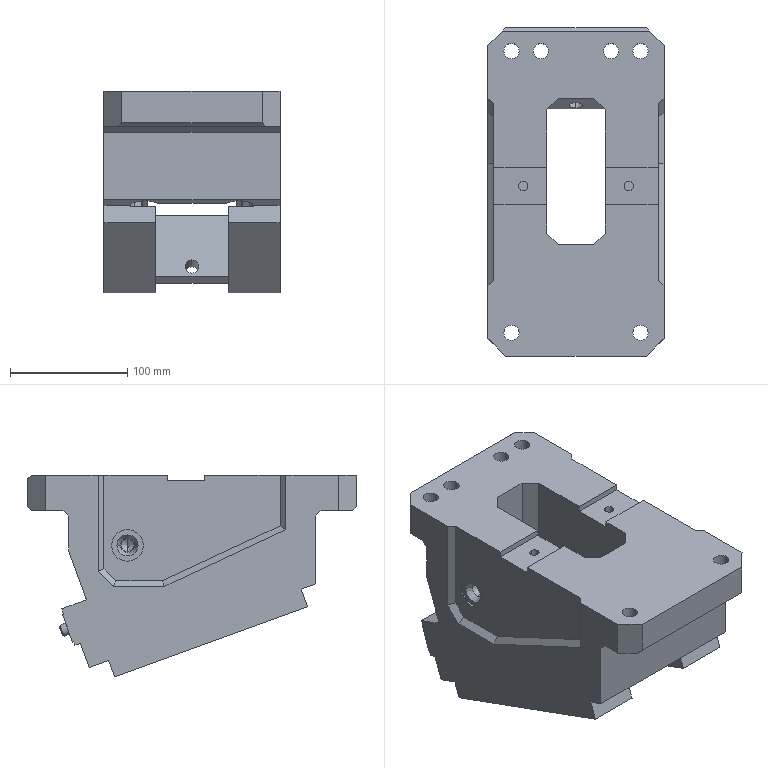Part | NX | features MEVN150-30_1;MEVN150-30_ASM|NEXT ASSEMBLY RELATIONSHIP#MGFV150-30_ASM|NEXT ASSEMBLY RELATIONSHIP#CAMHOLDER;CAMHOLDER 2 | 1 solid | 221 faces | box 150 x 280 x 172.066 mm | volume 2900097 mm3 | plane 149 | cylinder 48 | cone 12 | spline 12 | commonest cylinder face diameters 13 x12 20 x8 12 x6 8 x4 10 x4 10.4 x4